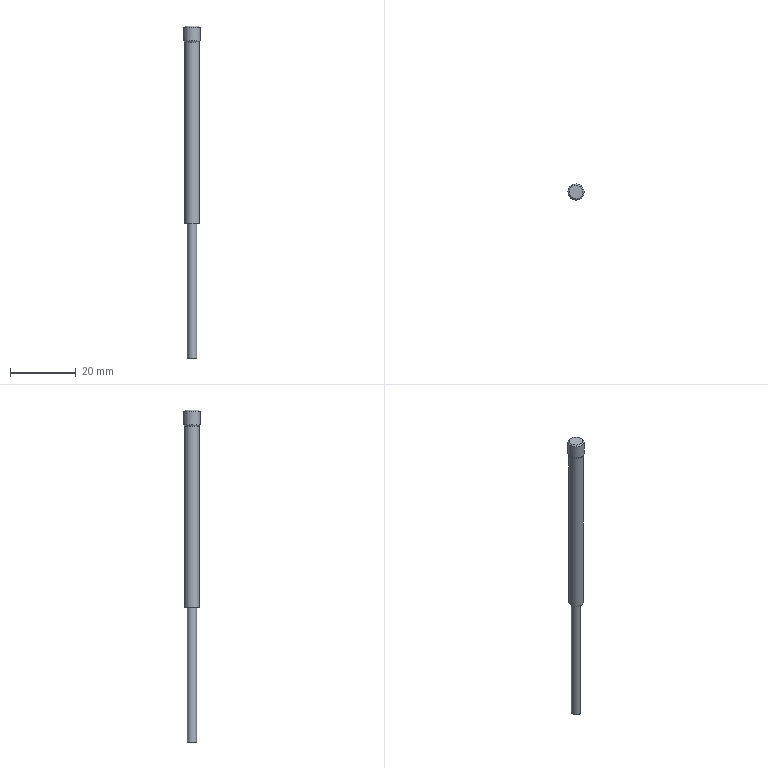Part | NX | features MI_APJEL_0257 2 | 1 solid | 9 faces | box 4.9 x 4.9 x 101 mm | volume 1181 mm3 | cylinder 3 | plane 3 | spline 2 | cone 1 | commonest cylinder face diameters 2.8 x1 4.4 x1 4.9 x1
STEP:
#1=CARTESIAN_POINT('',(1427.426,-30.228,73.1));
#2=VERTEX_POINT('',#1);
#3=CARTESIAN_POINT('',(1426.287,-34.478,73.1));
#4=VERTEX_POINT('',#3);
#5=CARTESIAN_POINT('',(1426.856,-32.353,73.1));
#6=DIRECTION('',(0.,0.,1.));
#7=DIRECTION('',(-0.2588,-0.9659,0.));
#8=AXIS2_PLACEMENT_3D('',#5,#6,#7);
#9=CIRCLE('',#8,2.2);
#10=EDGE_CURVE('',#2,#4,#9,.T.);
#11=ORIENTED_EDGE('',*,*,#10,.T.);
#12=CARTESIAN_POINT('',(1426.288,-34.479,73.1));
#13=VERTEX_POINT('',#12);
#14=CARTESIAN_POINT('',(1426.856,-32.353,73.1));
#15=DIRECTION('',(0.,0.,1.));
#16=DIRECTION('',(-0.2588,-0.9659,0.));
#17=AXIS2_PLACEMENT_3D('',#14,#15,#16);
#18=CIRCLE('',#17,2.2);
#19=EDGE_CURVE('',#4,#13,#18,.T.);
#20=ORIENTED_EDGE('',*,*,#19,.T.);
#21=CARTESIAN_POINT('',(1426.224,-34.72,73.448));
#22=VERTEX_POINT('',#21);
#23=CARTESIAN_POINT('',(1426.224,-34.72,73.448));
#24=DIRECTION('',(0.1505,0.5635,-0.8123));
#25=VECTOR('',#24,1000.);
#26=LINE('',#23,#25);
#27=EDGE_CURVE('',#22,#13,#26,.T.);
#28=ORIENTED_EDGE('',*,*,#27,.F.);
#29=CARTESIAN_POINT('',(1426.222,-34.72,73.448));
#30=VERTEX_POINT('',#29);
#31=CARTESIAN_POINT('',(1426.224,-34.72,73.448));
#32=CARTESIAN_POINT('',(1426.223,-34.72,73.448));
#33=CARTESIAN_POINT('',(1426.223,-34.72,73.448));
#34=CARTESIAN_POINT('',(1426.222,-34.72,73.448));
#35=B_SPLINE_CURVE_WITH_KNOTS('',3,(#31,#32,#33,#34),.UNSPECIFIED.,.F.,.F.,(4,4),(13.004,13.006),.UNSPECIFIED.);
#36=EDGE_CURVE('',#22,#30,#35,.T.);
#37=ORIENTED_EDGE('',*,*,#36,.T.);
#38=CARTESIAN_POINT('',(1424.495,-31.698,73.448));
#39=VERTEX_POINT('',#38);
#40=CARTESIAN_POINT('',(1426.222,-34.72,73.448));
#41=CARTESIAN_POINT('',(1425.917,-34.638,73.448));
#42=CARTESIAN_POINT('',(1425.622,-34.493,73.448));
#43=CARTESIAN_POINT('',(1425.12,-34.11,73.448));
#44=CARTESIAN_POINT('',(1424.902,-33.865,73.448));
#45=CARTESIAN_POINT('',(1424.583,-33.319,73.448));
#46=CARTESIAN_POINT('',(1424.475,-33.01,73.448));
#47=CARTESIAN_POINT('',(1424.386,-32.384,73.448));
#48=CARTESIAN_POINT('',(1424.404,-32.056,73.448));
#49=CARTESIAN_POINT('',(1424.486,-31.733,73.448));
#50=CARTESIAN_POINT('',(1424.491,-31.716,73.448));
#51=CARTESIAN_POINT('',(1424.495,-31.698,73.448));
#52=B_SPLINE_CURVE_WITH_KNOTS('',3,(#40,#41,#42,#43,#44,#45,#46,#47,#48,#49,#50,#51),.UNSPECIFIED.,.F.,.F.,(4,2,2,2,2,4),(0.,0.8058,1.612,2.418,3.223,3.269),.UNSPECIFIED.);
#53=EDGE_CURVE('',#30,#39,#52,.T.);
#54=ORIENTED_EDGE('',*,*,#53,.T.);
#55=CARTESIAN_POINT('',(1427.49,-29.987,73.448));
#56=VERTEX_POINT('',#55);
#57=CARTESIAN_POINT('',(1424.495,-31.698,73.448));
#58=CARTESIAN_POINT('',(1424.575,-31.41,73.448));
#59=CARTESIAN_POINT('',(1424.711,-31.133,73.448));
#60=CARTESIAN_POINT('',(1425.076,-30.64,73.448));
#61=CARTESIAN_POINT('',(1425.319,-30.419,73.448));
#62=CARTESIAN_POINT('',(1425.86,-30.092,73.448));
#63=CARTESIAN_POINT('',(1426.168,-29.98,73.448));
#64=CARTESIAN_POINT('',(1426.793,-29.884,73.448));
#65=CARTESIAN_POINT('',(1427.121,-29.897,73.448));
#66=CARTESIAN_POINT('',(1427.449,-29.976,73.448));
#67=CARTESIAN_POINT('',(1427.47,-29.981,73.448));
#68=CARTESIAN_POINT('',(1427.49,-29.987,73.448));
#69=B_SPLINE_CURVE_WITH_KNOTS('',3,(#57,#58,#59,#60,#61,#62,#63,#64,#65,#66,#67,#68),.UNSPECIFIED.,.F.,.F.,(4,2,2,2,2,4),(3.269,4.029,4.835,5.641,6.447,6.501),.UNSPECIFIED.);
#70=EDGE_CURVE('',#39,#56,#69,.T.);
#71=ORIENTED_EDGE('',*,*,#70,.T.);
#72=CARTESIAN_POINT('',(1427.425,-30.228,73.1));
#73=CARTESIAN_POINT('',(1427.447,-30.148,73.216));
#74=CARTESIAN_POINT('',(1427.469,-30.067,73.332));
#75=CARTESIAN_POINT('',(1427.49,-29.987,73.449));
#76=B_SPLINE_CURVE_WITH_KNOTS('',3,(#72,#73,#74,#75),.UNSPECIFIED.,.F.,.F.,(4,4),(0.,1.),.UNSPECIFIED.);
#77=EDGE_CURVE('',#2,#56,#76,.T.);
#78=ORIENTED_EDGE('',*,*,#77,.F.);
#79=EDGE_LOOP('',(#11,#20,#28,#37,#54,#71,#78));
#80=FACE_BOUND('',#79,.T.);
#81=CARTESIAN_POINT('',(1427.425,-30.228,73.1));
#82=CARTESIAN_POINT('',(1427.447,-30.148,73.216));
#83=CARTESIAN_POINT('',(1427.469,-30.067,73.332));
#84=CARTESIAN_POINT('',(1427.49,-29.987,73.449));
#85=CARTESIAN_POINT('',(1427.269,-30.187,73.1));
#86=CARTESIAN_POINT('',(1427.285,-30.104,73.216));
#87=CARTESIAN_POINT('',(1427.301,-30.022,73.332));
#88=CARTESIAN_POINT('',(1427.316,-29.94,73.449));
#89=CARTESIAN_POINT('',(1427.107,-30.162,73.1));
#90=CARTESIAN_POINT('',(1427.117,-30.079,73.216));
#91=CARTESIAN_POINT('',(1427.126,-29.996,73.332));
#92=CARTESIAN_POINT('',(1427.136,-29.913,73.449));
#93=CARTESIAN_POINT('',(1426.784,-30.149,73.1));
#94=CARTESIAN_POINT('',(1426.782,-30.065,73.216));
#95=CARTESIAN_POINT('',(1426.779,-29.982,73.332));
#96=CARTESIAN_POINT('',(1426.776,-29.898,73.449));
#97=CARTESIAN_POINT('',(1426.621,-30.16,73.1));
#98=CARTESIAN_POINT('',(1426.612,-30.077,73.216));
#99=CARTESIAN_POINT('',(1426.603,-29.994,73.332));
#100=CARTESIAN_POINT('',(1426.594,-29.911,73.449));
#101=CARTESIAN_POINT('',(1426.183,-30.24,73.1));
#102=CARTESIAN_POINT('',(1426.157,-30.16,73.216));
#103=CARTESIAN_POINT('',(1426.132,-30.08,73.332));
#104=CARTESIAN_POINT('',(1426.106,-30.,73.449));
#105=CARTESIAN_POINT('',(1425.909,-30.348,73.1));
#106=CARTESIAN_POINT('',(1425.873,-30.272,73.216));
#107=CARTESIAN_POINT('',(1425.837,-30.196,73.332));
#108=CARTESIAN_POINT('',(1425.801,-30.12,73.449));
#109=CARTESIAN_POINT('',(1425.431,-30.654,73.1));
#110=CARTESIAN_POINT('',(1425.377,-30.59,73.216));
#111=CARTESIAN_POINT('',(1425.323,-30.525,73.332));
#112=CARTESIAN_POINT('',(1425.269,-30.461,73.448));
#113=CARTESIAN_POINT('',(1425.218,-30.858,73.1));
#114=CARTESIAN_POINT('',(1425.156,-30.801,73.216));
#115=CARTESIAN_POINT('',(1425.094,-30.744,73.332));
#116=CARTESIAN_POINT('',(1425.032,-30.688,73.448));
#117=CARTESIAN_POINT('',(1424.892,-31.322,73.1));
#118=CARTESIAN_POINT('',(1424.818,-31.283,73.216));
#119=CARTESIAN_POINT('',(1424.743,-31.244,73.332));
#120=CARTESIAN_POINT('',(1424.669,-31.205,73.448));
#121=CARTESIAN_POINT('',(1424.773,-31.592,73.1));
#122=CARTESIAN_POINT('',(1424.694,-31.563,73.216));
#123=CARTESIAN_POINT('',(1424.615,-31.534,73.332));
#124=CARTESIAN_POINT('',(1424.536,-31.505,73.448));
#125=CARTESIAN_POINT('',(1424.648,-32.145,73.1));
#126=CARTESIAN_POINT('',(1424.564,-32.137,73.216));
#127=CARTESIAN_POINT('',(1424.481,-32.129,73.332));
#128=CARTESIAN_POINT('',(1424.397,-32.121,73.448));
#129=CARTESIAN_POINT('',(1424.64,-32.44,73.1));
#130=CARTESIAN_POINT('',(1424.556,-32.443,73.216));
#131=CARTESIAN_POINT('',(1424.472,-32.446,73.332));
#132=CARTESIAN_POINT('',(1424.388,-32.449,73.448));
#133=CARTESIAN_POINT('',(1424.734,-32.999,73.1));
#134=CARTESIAN_POINT('',(1424.654,-33.024,73.216));
#135=CARTESIAN_POINT('',(1424.573,-33.048,73.332));
#136=CARTESIAN_POINT('',(1424.493,-33.073,73.448));
#137=CARTESIAN_POINT('',(1424.838,-33.275,73.1));
#138=CARTESIAN_POINT('',(1424.762,-33.309,73.216));
#139=CARTESIAN_POINT('',(1424.685,-33.344,73.332));
#140=CARTESIAN_POINT('',(1424.609,-33.379,73.448));
#141=CARTESIAN_POINT('',(1425.138,-33.756,73.1));
#142=CARTESIAN_POINT('',(1425.073,-33.81,73.216));
#143=CARTESIAN_POINT('',(1425.008,-33.863,73.332));
#144=CARTESIAN_POINT('',(1424.943,-33.916,73.448));
#145=CARTESIAN_POINT('',(1425.339,-33.972,73.1));
#146=CARTESIAN_POINT('',(1425.282,-34.033,73.216));
#147=CARTESIAN_POINT('',(1425.224,-34.094,73.332));
#148=CARTESIAN_POINT('',(1425.167,-34.156,73.448));
#149=CARTESIAN_POINT('',(1425.799,-34.304,73.1));
#150=CARTESIAN_POINT('',(1425.759,-34.378,73.216));
#151=CARTESIAN_POINT('',(1425.719,-34.452,73.332));
#152=CARTESIAN_POINT('',(1425.679,-34.525,73.448));
#153=CARTESIAN_POINT('',(1426.067,-34.427,73.1));
#154=CARTESIAN_POINT('',(1426.037,-34.505,73.216));
#155=CARTESIAN_POINT('',(1426.007,-34.584,73.332));
#156=CARTESIAN_POINT('',(1425.977,-34.662,73.448));
#157=CARTESIAN_POINT('',(1426.619,-34.559,73.1));
#158=CARTESIAN_POINT('',(1426.61,-34.643,73.216));
#159=CARTESIAN_POINT('',(1426.601,-34.726,73.332));
#160=CARTESIAN_POINT('',(1426.592,-34.81,73.448));
#161=CARTESIAN_POINT('',(1426.913,-34.571,73.1));
#162=CARTESIAN_POINT('',(1426.915,-34.655,73.216));
#163=CARTESIAN_POINT('',(1426.918,-34.739,73.332));
#164=CARTESIAN_POINT('',(1426.92,-34.823,73.448));
#165=CARTESIAN_POINT('',(1427.474,-34.484,73.1));
#166=CARTESIAN_POINT('',(1427.497,-34.565,73.216));
#167=CARTESIAN_POINT('',(1427.521,-34.645,73.332));
#168=CARTESIAN_POINT('',(1427.544,-34.726,73.448));
#169=CARTESIAN_POINT('',(1427.751,-34.383,73.1));
#170=CARTESIAN_POINT('',(1427.785,-34.46,73.216));
#171=CARTESIAN_POINT('',(1427.819,-34.537,73.332));
#172=CARTESIAN_POINT('',(1427.852,-34.614,73.448));
#173=CARTESIAN_POINT('',(1428.237,-34.09,73.1));
#174=CARTESIAN_POINT('',(1428.289,-34.156,73.216));
#175=CARTESIAN_POINT('',(1428.341,-34.221,73.332));
#176=CARTESIAN_POINT('',(1428.393,-34.287,73.448));
#177=CARTESIAN_POINT('',(1428.454,-33.892,73.1));
#178=CARTESIAN_POINT('',(1428.515,-33.95,73.216));
#179=CARTESIAN_POINT('',(1428.576,-34.008,73.332));
#180=CARTESIAN_POINT('',(1428.636,-34.067,73.448));
#181=CARTESIAN_POINT('',(1428.792,-33.436,73.1));
#182=CARTESIAN_POINT('',(1428.866,-33.477,73.216));
#183=CARTESIAN_POINT('',(1428.939,-33.518,73.332));
#184=CARTESIAN_POINT('',(1429.013,-33.559,73.448));
#185=CARTESIAN_POINT('',(1428.919,-33.17,73.1));
#186=CARTESIAN_POINT('',(1428.997,-33.201,73.216));
#187=CARTESIAN_POINT('',(1429.075,-33.232,73.332));
#188=CARTESIAN_POINT('',(1429.153,-33.263,73.448));
#189=CARTESIAN_POINT('',(1429.058,-32.62,73.1));
#190=CARTESIAN_POINT('',(1429.142,-32.63,73.216));
#191=CARTESIAN_POINT('',(1429.225,-32.64,73.332));
#192=CARTESIAN_POINT('',(1429.309,-32.65,73.448));
#193=CARTESIAN_POINT('',(1429.074,-32.326,73.1));
#194=CARTESIAN_POINT('',(1429.158,-32.325,73.216));
#195=CARTESIAN_POINT('',(1429.242,-32.324,73.332));
#196=CARTESIAN_POINT('',(1429.326,-32.322,73.448));
#197=CARTESIAN_POINT('',(1428.995,-31.764,73.1));
#198=CARTESIAN_POINT('',(1429.076,-31.741,73.216));
#199=CARTESIAN_POINT('',(1429.157,-31.719,73.332));
#200=CARTESIAN_POINT('',(1429.238,-31.697,73.448));
#201=CARTESIAN_POINT('',(1428.898,-31.486,73.1));
#202=CARTESIAN_POINT('',(1428.975,-31.453,73.216));
#203=CARTESIAN_POINT('',(1429.052,-31.42,73.332));
#204=CARTESIAN_POINT('',(1429.13,-31.387,73.448));
#205=CARTESIAN_POINT('',(1428.611,-30.996,73.1));
#206=CARTESIAN_POINT('',(1428.677,-30.945,73.216));
#207=CARTESIAN_POINT('',(1428.744,-30.893,73.332));
#208=CARTESIAN_POINT('',(1428.81,-30.842,73.448));
#209=CARTESIAN_POINT('',(1428.415,-30.776,73.1));
#210=CARTESIAN_POINT('',(1428.474,-30.716,73.216));
#211=CARTESIAN_POINT('',(1428.533,-30.656,73.332));
#212=CARTESIAN_POINT('',(1428.592,-30.596,73.448));
#213=CARTESIAN_POINT('',(1427.964,-30.432,73.1));
#214=CARTESIAN_POINT('',(1428.006,-30.359,73.216));
#215=CARTESIAN_POINT('',(1428.048,-30.286,73.332));
#216=CARTESIAN_POINT('',(1428.09,-30.213,73.448));
#217=CARTESIAN_POINT('',(1427.7,-30.302,73.1));
#218=CARTESIAN_POINT('',(1427.731,-30.224,73.216));
#219=CARTESIAN_POINT('',(1427.763,-30.146,73.332));
#220=CARTESIAN_POINT('',(1427.795,-30.069,73.448));
#221=CARTESIAN_POINT('',(1427.425,-30.228,73.1));
#222=CARTESIAN_POINT('',(1427.447,-30.148,73.216));
#223=CARTESIAN_POINT('',(1427.469,-30.067,73.332));
#224=CARTESIAN_POINT('',(1427.49,-29.987,73.449));
#225=B_SPLINE_SURFACE_WITH_KNOTS('',3,3,((#81,#82,#83,#84),(#85,#86,#87,#88),(#89,#90,#91,#92),(#93,#94,#95,#96),(#97,#98,#99,#100),(#101,#102,#103,#104),(#105,#106,#107,#108),(#109,#110,#111,#112),(#113,#114,#115,#116),(#117,#118,#119,#120),(#121,#122,#123,#124),(#125,#126,#127,#128),(#129,#130,#131,#132),(#133,#134,#135,#136),(#137,#138,#139,#140),(#141,#142,#143,#144),(#145,#146,#147,#148),(#149,#150,#151,#152),(#153,#154,#155,#156),(#157,#158,#159,#160),(#161,#162,#163,#164),(#165,#166,#167,#168),(#169,#170,#171,#172),(#173,#174,#175,#176),(#177,#178,#179,#180),(#181,#182,#183,#184),(#185,#186,#187,#188),(#189,#190,#191,#192),(#193,#194,#195,#196),(#197,#198,#199,#200),(#201,#202,#203,#204),(#205,#206,#207,#208),(#209,#210,#211,#212),(#213,#214,#215,#216),(#217,#218,#219,#220),(#221,#222,#223,#224)),.RULED_SURF.,.T.,.F.,.F.,(4,2,2,2,2,2,2,2,2,2,2,2,2,2,2,2,2,4),(4,4),(-13.006,-12.547,-12.088,-11.282,-10.476,-9.67,-8.864,-8.058,-7.253,-6.447,-5.641,-4.835,-4.029,-3.223,-2.418,-1.612,-0.8058,0.),(0.,1.),.UNSPECIFIED.);
#226=ADVANCED_FACE('',(#80),#225,.T.);
#227=CARTESIAN_POINT('',(1426.208,-34.716,77.632));
#228=VERTEX_POINT('',#227);
#229=CARTESIAN_POINT('',(1427.49,-29.987,77.632));
#230=VERTEX_POINT('',#229);
#231=CARTESIAN_POINT('',(1426.856,-32.353,77.632));
#232=DIRECTION('',(0.,0.,1.));
#233=DIRECTION('',(0.2588,0.9659,0.));
#234=AXIS2_PLACEMENT_3D('',#231,#232,#233);
#235=CIRCLE('',#234,2.45);
#236=EDGE_CURVE('',#228,#230,#235,.T.);
#237=ORIENTED_EDGE('',*,*,#236,.F.);
#238=CARTESIAN_POINT('',(1424.495,-31.698,77.632));
#239=VERTEX_POINT('',#238);
#240=CARTESIAN_POINT('',(1426.856,-32.353,77.632));
#241=DIRECTION('',(0.,0.,1.));
#242=DIRECTION('',(0.2588,0.9659,0.));
#243=AXIS2_PLACEMENT_3D('',#240,#241,#242);
#244=CIRCLE('',#243,2.45);
#245=EDGE_CURVE('',#239,#228,#244,.T.);
#246=ORIENTED_EDGE('',*,*,#245,.F.);
#247=CARTESIAN_POINT('',(1424.495,-31.698,77.632));
#248=CARTESIAN_POINT('',(1424.495,-31.698,73.448));
#249=B_SPLINE_CURVE_WITH_KNOTS('',1,(#247,#248),.UNSPECIFIED.,.F.,.F.,(2,2),(0.08333,0.9167),.UNSPECIFIED.);
#250=EDGE_CURVE('',#239,#39,#249,.T.);
#251=ORIENTED_EDGE('',*,*,#250,.T.);
#252=ORIENTED_EDGE('',*,*,#53,.F.);
#253=ORIENTED_EDGE('',*,*,#36,.F.);
#254=CARTESIAN_POINT('',(1427.49,-29.987,73.448));
#255=CARTESIAN_POINT('',(1427.775,-30.063,73.448));
#256=CARTESIAN_POINT('',(1428.051,-30.194,73.448));
#257=CARTESIAN_POINT('',(1428.546,-30.551,73.448));
#258=CARTESIAN_POINT('',(1428.77,-30.791,73.448));
#259=CARTESIAN_POINT('',(1429.104,-31.327,73.448));
#260=CARTESIAN_POINT('',(1429.22,-31.634,73.448));
#261=CARTESIAN_POINT('',(1429.325,-32.257,73.448));
#262=CARTESIAN_POINT('',(1429.316,-32.585,73.448));
#263=CARTESIAN_POINT('',(1429.176,-33.202,73.448));
#264=CARTESIAN_POINT('',(1429.043,-33.502,73.448));
#265=CARTESIAN_POINT('',(1428.68,-34.019,73.448));
#266=CARTESIAN_POINT('',(1428.443,-34.246,73.448));
#267=CARTESIAN_POINT('',(1427.911,-34.587,73.448));
#268=CARTESIAN_POINT('',(1427.606,-34.707,73.448));
#269=CARTESIAN_POINT('',(1427.118,-34.796,73.448));
#270=CARTESIAN_POINT('',(1426.936,-34.808,73.448));
#271=CARTESIAN_POINT('',(1426.577,-34.794,73.448));
#272=CARTESIAN_POINT('',(1426.397,-34.766,73.448));
#273=CARTESIAN_POINT('',(1426.224,-34.72,73.448));
#274=B_SPLINE_CURVE_WITH_KNOTS('',3,(#254,#255,#256,#257,#258,#259,#260,#261,#262,#263,#264,#265,#266,#267,#268,#269,#270,#271,#272,#273),.UNSPECIFIED.,.F.,.F.,(4,2,2,2,2,2,2,2,2,4),(6.501,7.253,8.058,8.864,9.67,10.476,11.282,12.088,12.547,13.004),.UNSPECIFIED.);
#275=EDGE_CURVE('',#56,#22,#274,.T.);
#276=ORIENTED_EDGE('',*,*,#275,.F.);
#277=ORIENTED_EDGE('',*,*,#70,.F.);
#278=ORIENTED_EDGE('',*,*,#250,.F.);
#279=CARTESIAN_POINT('',(1426.856,-32.353,77.632));
#280=DIRECTION('',(0.,0.,1.));
#281=DIRECTION('',(0.2588,0.9659,0.));
#282=AXIS2_PLACEMENT_3D('',#279,#280,#281);
#283=CIRCLE('',#282,2.45);
#284=EDGE_CURVE('',#230,#239,#283,.T.);
#285=ORIENTED_EDGE('',*,*,#284,.F.);
#286=EDGE_LOOP('',(#237,#246,#251,#252,#253,#276,#277,#278,#285));
#287=FACE_BOUND('',#286,.T.);
#288=CARTESIAN_POINT('',(1426.856,-32.353,75.55));
#289=DIRECTION('',(0.,0.,-1.));
#290=DIRECTION('',(-0.9636,0.2672,0.));
#291=AXIS2_PLACEMENT_3D('',#288,#289,#290);
#292=CYLINDRICAL_SURFACE('',#291,2.45);
#293=ADVANCED_FACE('',(#287),#292,.T.);
#294=CARTESIAN_POINT('',(1427.395,-30.342,78.));
#295=VERTEX_POINT('',#294);
#296=CARTESIAN_POINT('',(1426.305,-34.361,78.));
#297=VERTEX_POINT('',#296);
#298=CARTESIAN_POINT('',(1426.856,-32.353,78.));
#299=DIRECTION('',(0.,0.,-1.));
#300=DIRECTION('',(0.2588,0.9659,0.));
#301=AXIS2_PLACEMENT_3D('',#298,#299,#300);
#302=CIRCLE('',#301,2.083);
#303=EDGE_CURVE('',#295,#297,#302,.T.);
#304=ORIENTED_EDGE('',*,*,#303,.T.);
#305=CARTESIAN_POINT('',(1426.305,-34.361,78.));
#306=CARTESIAN_POINT('',(1426.208,-34.716,77.633));
#307=B_SPLINE_CURVE_WITH_KNOTS('',1,(#305,#306),.UNSPECIFIED.,.F.,.F.,(2,2),(0.601,0.7071),.UNSPECIFIED.);
#308=EDGE_CURVE('',#297,#228,#307,.T.);
#309=ORIENTED_EDGE('',*,*,#308,.T.);
#310=ORIENTED_EDGE('',*,*,#236,.T.);
#311=ORIENTED_EDGE('',*,*,#284,.T.);
#312=ORIENTED_EDGE('',*,*,#245,.T.);
#313=ORIENTED_EDGE('',*,*,#308,.F.);
#314=CARTESIAN_POINT('',(1426.856,-32.353,78.));
#315=DIRECTION('',(0.,0.,-1.));
#316=DIRECTION('',(0.2588,0.9659,0.));
#317=AXIS2_PLACEMENT_3D('',#314,#315,#316);
#318=CIRCLE('',#317,2.083);
#319=EDGE_CURVE('',#297,#295,#318,.T.);
#320=ORIENTED_EDGE('',*,*,#319,.T.);
#321=EDGE_LOOP('',(#304,#309,#310,#311,#312,#313,#320));
#322=FACE_BOUND('',#321,.T.);
#323=CARTESIAN_POINT('',(1426.856,-32.353,76.618));
#324=DIRECTION('',(0.,0.,-1.));
#325=DIRECTION('',(-0.2644,-0.9644,0.));
#326=AXIS2_PLACEMENT_3D('',#323,#324,#325);
#327=CONICAL_SURFACE('',#326,3.465,0.7854);
#328=ADVANCED_FACE('',(#322),#327,.T.);
#329=ORIENTED_EDGE('',*,*,#319,.F.);
#330=ORIENTED_EDGE('',*,*,#303,.F.);
#331=EDGE_LOOP('',(#329,#330));
#332=FACE_BOUND('',#331,.T.);
#333=CARTESIAN_POINT('',(1423.376,-28.618,78.));
#334=DIRECTION('',(0.,0.,1.));
#335=DIRECTION('',(-0.2588,-0.9659,0.));
#336=AXIS2_PLACEMENT_3D('',#333,#334,#335);
#337=PLANE('',#336);
#338=ADVANCED_FACE('',(#332),#337,.T.);
#339=CARTESIAN_POINT('',(1427.219,-31.001,18.));
#340=VERTEX_POINT('',#339);
#341=CARTESIAN_POINT('',(1426.856,-32.353,18.));
#342=DIRECTION('',(0.,0.,1.));
#343=DIRECTION('',(0.2588,0.9659,0.));
#344=AXIS2_PLACEMENT_3D('',#341,#342,#343);
#345=CIRCLE('',#344,1.4);
#346=EDGE_CURVE('',#340,#340,#345,.T.);
#347=ORIENTED_EDGE('',*,*,#346,.F.);
#348=CARTESIAN_POINT('',(1427.219,-31.001,-23.));
#349=VERTEX_POINT('',#348);
#350=CARTESIAN_POINT('',(1427.219,-31.001,18.));
#351=CARTESIAN_POINT('',(1427.219,-31.001,-23.));
#352=B_SPLINE_CURVE_WITH_KNOTS('',1,(#350,#351),.UNSPECIFIED.,.F.,.F.,(2,2),(0.08333,0.9167),.UNSPECIFIED.);
#353=EDGE_CURVE('',#340,#349,#352,.T.);
#354=ORIENTED_EDGE('',*,*,#353,.T.);
#355=CARTESIAN_POINT('',(1426.856,-32.353,-23.));
#356=DIRECTION('',(0.,0.,-1.));
#357=DIRECTION('',(0.2588,0.9659,0.));
#358=AXIS2_PLACEMENT_3D('',#355,#356,#357);
#359=CIRCLE('',#358,1.4);
#360=EDGE_CURVE('',#349,#349,#359,.T.);
#361=ORIENTED_EDGE('',*,*,#360,.F.);
#362=ORIENTED_EDGE('',*,*,#353,.F.);
#363=EDGE_LOOP('',(#347,#354,#361,#362));
#364=FACE_BOUND('',#363,.T.);
#365=CARTESIAN_POINT('',(1426.856,-32.353,-2.5));
#366=DIRECTION('',(0.,0.,-1.));
#367=DIRECTION('',(0.2588,0.9659,0.));
#368=AXIS2_PLACEMENT_3D('',#365,#366,#367);
#369=CYLINDRICAL_SURFACE('',#368,1.4);
#370=ADVANCED_FACE('',(#364),#369,.T.);
#371=ORIENTED_EDGE('',*,*,#360,.T.);
#372=EDGE_LOOP('',(#371));
#373=FACE_BOUND('',#372,.T.);
#374=CARTESIAN_POINT('',(1423.212,-34.71,-23.));
#375=DIRECTION('',(0.,0.,-1.));
#376=DIRECTION('',(0.2588,0.9659,0.));
#377=AXIS2_PLACEMENT_3D('',#374,#375,#376);
#378=PLANE('',#377);
#379=ADVANCED_FACE('',(#373),#378,.T.);
#380=ORIENTED_EDGE('',*,*,#10,.F.);
#381=CARTESIAN_POINT('',(1427.426,-30.228,18.));
#382=VERTEX_POINT('',#381);
#383=CARTESIAN_POINT('',(1427.426,-30.228,73.1));
#384=CARTESIAN_POINT('',(1427.426,-30.228,18.));
#385=B_SPLINE_CURVE_WITH_KNOTS('',1,(#383,#384),.UNSPECIFIED.,.F.,.F.,(2,2),(0.08333,0.9167),.UNSPECIFIED.);
#386=EDGE_CURVE('',#2,#382,#385,.T.);
#387=ORIENTED_EDGE('',*,*,#386,.T.);
#388=CARTESIAN_POINT('',(1426.856,-32.353,18.));
#389=DIRECTION('',(0.,0.,-1.));
#390=DIRECTION('',(0.2588,0.9659,0.));
#391=AXIS2_PLACEMENT_3D('',#388,#389,#390);
#392=CIRCLE('',#391,2.2);
#393=EDGE_CURVE('',#382,#382,#392,.T.);
#394=ORIENTED_EDGE('',*,*,#393,.F.);
#395=ORIENTED_EDGE('',*,*,#386,.F.);
#396=CARTESIAN_POINT('',(1426.856,-32.353,73.1));
#397=DIRECTION('',(0.,0.,1.));
#398=DIRECTION('',(-0.2588,-0.9659,0.));
#399=AXIS2_PLACEMENT_3D('',#396,#397,#398);
#400=CIRCLE('',#399,2.2);
#401=EDGE_CURVE('',#13,#2,#400,.T.);
#402=ORIENTED_EDGE('',*,*,#401,.F.);
#403=ORIENTED_EDGE('',*,*,#19,.F.);
#404=EDGE_LOOP('',(#380,#387,#394,#395,#402,#403));
#405=FACE_BOUND('',#404,.T.);
#406=CARTESIAN_POINT('',(1426.856,-32.353,45.55));
#407=DIRECTION('',(0.,0.,-1.));
#408=DIRECTION('',(0.2588,0.9659,0.));
#409=AXIS2_PLACEMENT_3D('',#406,#407,#408);
#410=CYLINDRICAL_SURFACE('',#409,2.2);
#411=ADVANCED_FACE('',(#405),#410,.T.);
#412=ORIENTED_EDGE('',*,*,#393,.T.);
#413=EDGE_LOOP('',(#412));
#414=FACE_BOUND('',#413,.T.);
#415=ORIENTED_EDGE('',*,*,#346,.T.);
#416=EDGE_LOOP('',(#415));
#417=FACE_BOUND('',#416,.T.);
#418=CARTESIAN_POINT('',(1421.13,-36.057,18.));
#419=DIRECTION('',(0.,0.,-1.));
#420=DIRECTION('',(0.2588,0.9659,0.));
#421=AXIS2_PLACEMENT_3D('',#418,#419,#420);
#422=PLANE('',#421);
#423=ADVANCED_FACE('',(#414,#417),#422,.T.);
#424=ORIENTED_EDGE('',*,*,#275,.T.);
#425=ORIENTED_EDGE('',*,*,#27,.T.);
#426=ORIENTED_EDGE('',*,*,#401,.T.);
#427=ORIENTED_EDGE('',*,*,#77,.T.);
#428=EDGE_LOOP('',(#424,#425,#426,#427));
#429=FACE_BOUND('',#428,.T.);
#430=CARTESIAN_POINT('',(1427.425,-30.228,73.1));
#431=CARTESIAN_POINT('',(1427.447,-30.148,73.216));
#432=CARTESIAN_POINT('',(1427.469,-30.067,73.332));
#433=CARTESIAN_POINT('',(1427.49,-29.987,73.449));
#434=CARTESIAN_POINT('',(1427.269,-30.187,73.1));
#435=CARTESIAN_POINT('',(1427.285,-30.104,73.216));
#436=CARTESIAN_POINT('',(1427.301,-30.022,73.332));
#437=CARTESIAN_POINT('',(1427.316,-29.94,73.449));
#438=CARTESIAN_POINT('',(1427.107,-30.162,73.1));
#439=CARTESIAN_POINT('',(1427.117,-30.079,73.216));
#440=CARTESIAN_POINT('',(1427.126,-29.996,73.332));
#441=CARTESIAN_POINT('',(1427.136,-29.913,73.449));
#442=CARTESIAN_POINT('',(1426.784,-30.149,73.1));
#443=CARTESIAN_POINT('',(1426.782,-30.065,73.216));
#444=CARTESIAN_POINT('',(1426.779,-29.982,73.332));
#445=CARTESIAN_POINT('',(1426.776,-29.898,73.449));
#446=CARTESIAN_POINT('',(1426.621,-30.16,73.1));
#447=CARTESIAN_POINT('',(1426.612,-30.077,73.216));
#448=CARTESIAN_POINT('',(1426.603,-29.994,73.332));
#449=CARTESIAN_POINT('',(1426.594,-29.911,73.449));
#450=CARTESIAN_POINT('',(1426.183,-30.24,73.1));
#451=CARTESIAN_POINT('',(1426.157,-30.16,73.216));
#452=CARTESIAN_POINT('',(1426.132,-30.08,73.332));
#453=CARTESIAN_POINT('',(1426.106,-30.,73.449));
#454=CARTESIAN_POINT('',(1425.909,-30.348,73.1));
#455=CARTESIAN_POINT('',(1425.873,-30.272,73.216));
#456=CARTESIAN_POINT('',(1425.837,-30.196,73.332));
#457=CARTESIAN_POINT('',(1425.801,-30.12,73.449));
#458=CARTESIAN_POINT('',(1425.431,-30.654,73.1));
#459=CARTESIAN_POINT('',(1425.377,-30.59,73.216));
#460=CARTESIAN_POINT('',(1425.323,-30.525,73.332));
#461=CARTESIAN_POINT('',(1425.269,-30.461,73.448));
#462=CARTESIAN_POINT('',(1425.218,-30.858,73.1));
#463=CARTESIAN_POINT('',(1425.156,-30.801,73.216));
#464=CARTESIAN_POINT('',(1425.094,-30.744,73.332));
#465=CARTESIAN_POINT('',(1425.032,-30.688,73.448));
#466=CARTESIAN_POINT('',(1424.892,-31.322,73.1));
#467=CARTESIAN_POINT('',(1424.818,-31.283,73.216));
#468=CARTESIAN_POINT('',(1424.743,-31.244,73.332));
#469=CARTESIAN_POINT('',(1424.669,-31.205,73.448));
#470=CARTESIAN_POINT('',(1424.773,-31.592,73.1));
#471=CARTESIAN_POINT('',(1424.694,-31.563,73.216));
#472=CARTESIAN_POINT('',(1424.615,-31.534,73.332));
#473=CARTESIAN_POINT('',(1424.536,-31.505,73.448));
#474=CARTESIAN_POINT('',(1424.648,-32.145,73.1));
#475=CARTESIAN_POINT('',(1424.564,-32.137,73.216));
#476=CARTESIAN_POINT('',(1424.481,-32.129,73.332));
#477=CARTESIAN_POINT('',(1424.397,-32.121,73.448));
#478=CARTESIAN_POINT('',(1424.64,-32.44,73.1));
#479=CARTESIAN_POINT('',(1424.556,-32.443,73.216));
#480=CARTESIAN_POINT('',(1424.472,-32.446,73.332));
#481=CARTESIAN_POINT('',(1424.388,-32.449,73.448));
#482=CARTESIAN_POINT('',(1424.734,-32.999,73.1));
#483=CARTESIAN_POINT('',(1424.654,-33.024,73.216));
#484=CARTESIAN_POINT('',(1424.573,-33.048,73.332));
#485=CARTESIAN_POINT('',(1424.493,-33.073,73.448));
#486=CARTESIAN_POINT('',(1424.838,-33.275,73.1));
#487=CARTESIAN_POINT('',(1424.762,-33.309,73.216));
#488=CARTESIAN_POINT('',(1424.685,-33.344,73.332));
#489=CARTESIAN_POINT('',(1424.609,-33.379,73.448));
#490=CARTESIAN_POINT('',(1425.138,-33.756,73.1));
#491=CARTESIAN_POINT('',(1425.073,-33.81,73.216));
#492=CARTESIAN_POINT('',(1425.008,-33.863,73.332));
#493=CARTESIAN_POINT('',(1424.943,-33.916,73.448));
#494=CARTESIAN_POINT('',(1425.339,-33.972,73.1));
#495=CARTESIAN_POINT('',(1425.282,-34.033,73.216));
#496=CARTESIAN_POINT('',(1425.224,-34.094,73.332));
#497=CARTESIAN_POINT('',(1425.167,-34.156,73.448));
#498=CARTESIAN_POINT('',(1425.799,-34.304,73.1));
#499=CARTESIAN_POINT('',(1425.759,-34.378,73.216));
#500=CARTESIAN_POINT('',(1425.719,-34.452,73.332));
#501=CARTESIAN_POINT('',(1425.679,-34.525,73.448));
#502=CARTESIAN_POINT('',(1426.067,-34.427,73.1));
#503=CARTESIAN_POINT('',(1426.037,-34.505,73.216));
#504=CARTESIAN_POINT('',(1426.007,-34.584,73.332));
#505=CARTESIAN_POINT('',(1425.977,-34.662,73.448));
#506=CARTESIAN_POINT('',(1426.619,-34.559,73.1));
#507=CARTESIAN_POINT('',(1426.61,-34.643,73.216));
#508=CARTESIAN_POINT('',(1426.601,-34.726,73.332));
#509=CARTESIAN_POINT('',(1426.592,-34.81,73.448));
#510=CARTESIAN_POINT('',(1426.913,-34.571,73.1));
#511=CARTESIAN_POINT('',(1426.915,-34.655,73.216));
#512=CARTESIAN_POINT('',(1426.918,-34.739,73.332));
#513=CARTESIAN_POINT('',(1426.92,-34.823,73.448));
#514=CARTESIAN_POINT('',(1427.474,-34.484,73.1));
#515=CARTESIAN_POINT('',(1427.497,-34.565,73.216));
#516=CARTESIAN_POINT('',(1427.521,-34.645,73.332));
#517=CARTESIAN_POINT('',(1427.544,-34.726,73.448));
#518=CARTESIAN_POINT('',(1427.751,-34.383,73.1));
#519=CARTESIAN_POINT('',(1427.785,-34.46,73.216));
#520=CARTESIAN_POINT('',(1427.819,-34.537,73.332));
#521=CARTESIAN_POINT('',(1427.852,-34.614,73.448));
#522=CARTESIAN_POINT('',(1428.237,-34.09,73.1));
#523=CARTESIAN_POINT('',(1428.289,-34.156,73.216));
#524=CARTESIAN_POINT('',(1428.341,-34.221,73.332));
#525=CARTESIAN_POINT('',(1428.393,-34.287,73.448));
#526=CARTESIAN_POINT('',(1428.454,-33.892,73.1));
#527=CARTESIAN_POINT('',(1428.515,-33.95,73.216));
#528=CARTESIAN_POINT('',(1428.576,-34.008,73.332));
#529=CARTESIAN_POINT('',(1428.636,-34.067,73.448));
#530=CARTESIAN_POINT('',(1428.792,-33.436,73.1));
#531=CARTESIAN_POINT('',(1428.866,-33.477,73.216));
#532=CARTESIAN_POINT('',(1428.939,-33.518,73.332));
#533=CARTESIAN_POINT('',(1429.013,-33.559,73.448));
#534=CARTESIAN_POINT('',(1428.919,-33.17,73.1));
#535=CARTESIAN_POINT('',(1428.997,-33.201,73.216));
#536=CARTESIAN_POINT('',(1429.075,-33.232,73.332));
#537=CARTESIAN_POINT('',(1429.153,-33.263,73.448));
#538=CARTESIAN_POINT('',(1429.058,-32.62,73.1));
#539=CARTESIAN_POINT('',(1429.142,-32.63,73.216));
#540=CARTESIAN_POINT('',(1429.225,-32.64,73.332));
#541=CARTESIAN_POINT('',(1429.309,-32.65,73.448));
#542=CARTESIAN_POINT('',(1429.074,-32.326,73.1));
#543=CARTESIAN_POINT('',(1429.158,-32.325,73.216));
#544=CARTESIAN_POINT('',(1429.242,-32.324,73.332));
#545=CARTESIAN_POINT('',(1429.326,-32.322,73.448));
#546=CARTESIAN_POINT('',(1428.995,-31.764,73.1));
#547=CARTESIAN_POINT('',(1429.076,-31.741,73.216));
#548=CARTESIAN_POINT('',(1429.157,-31.719,73.332));
#549=CARTESIAN_POINT('',(1429.238,-31.697,73.448));
#550=CARTESIAN_POINT('',(1428.898,-31.486,73.1));
#551=CARTESIAN_POINT('',(1428.975,-31.453,73.216));
#552=CARTESIAN_POINT('',(1429.052,-31.42,73.332));
#553=CARTESIAN_POINT('',(1429.13,-31.387,73.448));
#554=CARTESIAN_POINT('',(1428.611,-30.996,73.1));
#555=CARTESIAN_POINT('',(1428.677,-30.945,73.216));
#556=CARTESIAN_POINT('',(1428.744,-30.893,73.332));
#557=CARTESIAN_POINT('',(1428.81,-30.842,73.448));
#558=CARTESIAN_POINT('',(1428.415,-30.776,73.1));
#559=CARTESIAN_POINT('',(1428.474,-30.716,73.216));
#560=CARTESIAN_POINT('',(1428.533,-30.656,73.332));
#561=CARTESIAN_POINT('',(1428.592,-30.596,73.448));
#562=CARTESIAN_POINT('',(1427.964,-30.432,73.1));
#563=CARTESIAN_POINT('',(1428.006,-30.359,73.216));
#564=CARTESIAN_POINT('',(1428.048,-30.286,73.332));
#565=CARTESIAN_POINT('',(1428.09,-30.213,73.448));
#566=CARTESIAN_POINT('',(1427.7,-30.302,73.1));
#567=CARTESIAN_POINT('',(1427.731,-30.224,73.216));
#568=CARTESIAN_POINT('',(1427.763,-30.146,73.332));
#569=CARTESIAN_POINT('',(1427.795,-30.069,73.448));
#570=CARTESIAN_POINT('',(1427.425,-30.228,73.1));
#571=CARTESIAN_POINT('',(1427.447,-30.148,73.216));
#572=CARTESIAN_POINT('',(1427.469,-30.067,73.332));
#573=CARTESIAN_POINT('',(1427.49,-29.987,73.449));
#574=B_SPLINE_SURFACE_WITH_KNOTS('',3,3,((#430,#431,#432,#433),(#434,#435,#436,#437),(#438,#439,#440,#441),(#442,#443,#444,#445),(#446,#447,#448,#449),(#450,#451,#452,#453),(#454,#455,#456,#457),(#458,#459,#460,#461),(#462,#463,#464,#465),(#466,#467,#468,#469),(#470,#471,#472,#473),(#474,#475,#476,#477),(#478,#479,#480,#481),(#482,#483,#484,#485),(#486,#487,#488,#489),(#490,#491,#492,#493),(#494,#495,#496,#497),(#498,#499,#500,#501),(#502,#503,#504,#505),(#506,#507,#508,#509),(#510,#511,#512,#513),(#514,#515,#516,#517),(#518,#519,#520,#521),(#522,#523,#524,#525),(#526,#527,#528,#529),(#530,#531,#532,#533),(#534,#535,#536,#537),(#538,#539,#540,#541),(#542,#543,#544,#545),(#546,#547,#548,#549),(#550,#551,#552,#553),(#554,#555,#556,#557),(#558,#559,#560,#561),(#562,#563,#564,#565),(#566,#567,#568,#569),(#570,#571,#572,#573)),.RULED_SURF.,.T.,.F.,.F.,(4,2,2,2,2,2,2,2,2,2,2,2,2,2,2,2,2,4),(4,4),(-13.006,-12.547,-12.088,-11.282,-10.476,-9.67,-8.864,-8.058,-7.253,-6.447,-5.641,-4.835,-4.029,-3.223,-2.418,-1.612,-0.8058,0.),(0.,1.),.UNSPECIFIED.);
#575=ADVANCED_FACE('',(#429),#574,.T.);
#576=CLOSED_SHELL('',(#226,#293,#328,#338,#370,#379,#411,#423,#575));
#577=MANIFOLD_SOLID_BREP('',#576);
#578=(LENGTH_UNIT()NAMED_UNIT(*)SI_UNIT(.MILLI.,.METRE.));
#579=UNCERTAINTY_MEASURE_WITH_UNIT(LENGTH_MEASURE(0.00001),#578,'','');
#580=(NAMED_UNIT(*)PLANE_ANGLE_UNIT()SI_UNIT($,.RADIAN.));
#581=(NAMED_UNIT(*)SI_UNIT($,.STERADIAN.)SOLID_ANGLE_UNIT());
#582=(GEOMETRIC_REPRESENTATION_CONTEXT(3)GLOBAL_UNCERTAINTY_ASSIGNED_CONTEXT((#579))GLOBAL_UNIT_ASSIGNED_CONTEXT((#578,#580,#581))REPRESENTATION_CONTEXT('',''));
#583=ADVANCED_BREP_SHAPE_REPRESENTATION('',(#577),#582);